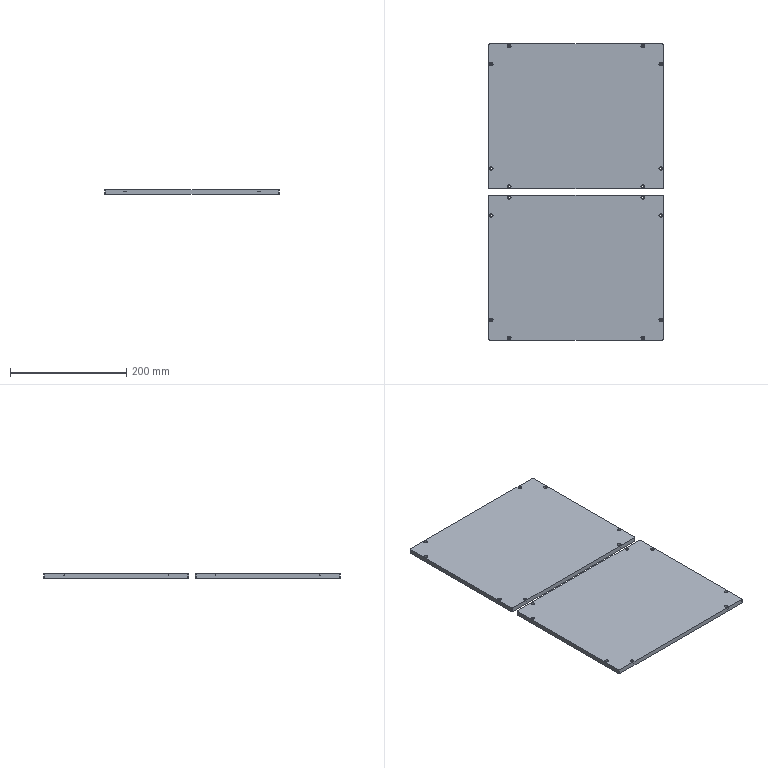Part | 2 solids | 100 faces | box 300 x 511 x 8 mm | volume 1197693 mm3 | cylinder 72 | plane 28 | commonest cylinder face diameters 3.5 x32 6 x32 3 x8